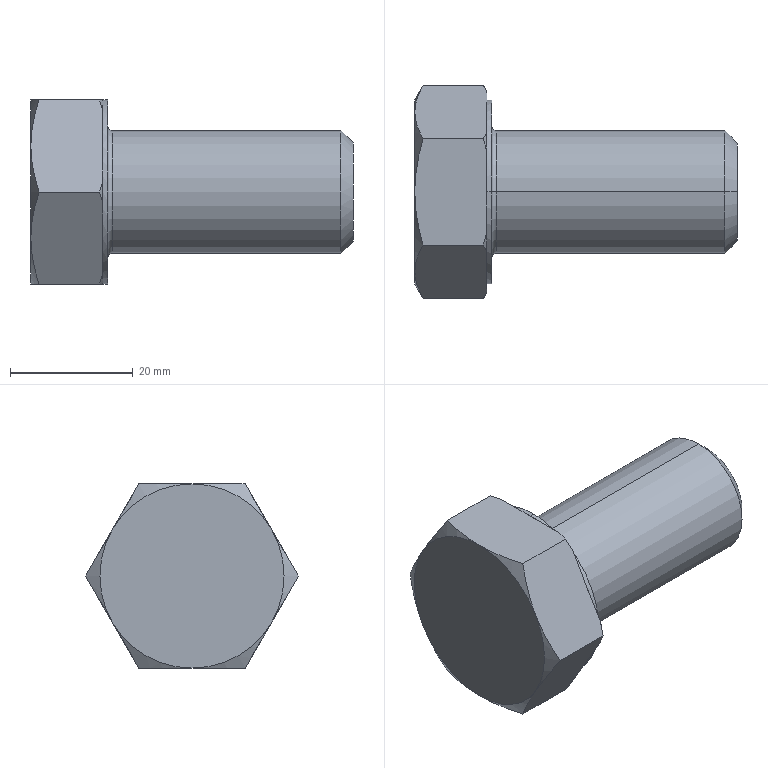Part | SolidWorks | 1 solid | 35 faces | box 52.5 x 34.641 x 30 mm | volume 22112 mm3 | plane 15 | cone 14 | cylinder 4 | torus 2 | commonest cylinder face diameters 20 x2 30 x2
STEP:
#1=CARTESIAN_POINT('',(13.3,0.,10.));
#2=VERTEX_POINT('',#1);
#3=CARTESIAN_POINT('',(13.3,0.,-10.));
#4=VERTEX_POINT('',#3);
#5=CARTESIAN_POINT('',(13.3,0.,0.));
#6=DIRECTION('',(1.,0.,0.));
#7=DIRECTION('',(0.,0.,-1.));
#8=AXIS2_PLACEMENT_3D('',#5,#6,#7);
#9=CIRCLE('',#8,10.);
#10=EDGE_CURVE('',#2,#4,#9,.T.);
#11=ORIENTED_EDGE('',*,*,#10,.F.);
#12=CARTESIAN_POINT('',(12.5,0.,10.8));
#13=VERTEX_POINT('',#12);
#14=CARTESIAN_POINT('',(13.3,0.,10.8));
#15=DIRECTION('',(0.,1.,0.));
#16=DIRECTION('',(0.,0.,1.));
#17=AXIS2_PLACEMENT_3D('',#14,#15,#16);
#18=CIRCLE('',#17,0.8);
#19=EDGE_CURVE('',#2,#13,#18,.T.);
#20=ORIENTED_EDGE('',*,*,#19,.T.);
#21=CARTESIAN_POINT('',(12.5,0.,-10.8));
#22=VERTEX_POINT('',#21);
#23=CARTESIAN_POINT('',(12.5,0.,0.));
#24=DIRECTION('',(-1.,0.,0.));
#25=DIRECTION('',(0.,0.,-1.));
#26=AXIS2_PLACEMENT_3D('',#23,#24,#25);
#27=CIRCLE('',#26,10.8);
#28=EDGE_CURVE('',#22,#13,#27,.T.);
#29=ORIENTED_EDGE('',*,*,#28,.F.);
#30=CARTESIAN_POINT('',(13.3,0.,-10.8));
#31=DIRECTION('',(0.,-1.,0.));
#32=DIRECTION('',(0.,0.,-1.));
#33=AXIS2_PLACEMENT_3D('',#30,#31,#32);
#34=CIRCLE('',#33,0.8);
#35=EDGE_CURVE('',#4,#22,#34,.T.);
#36=ORIENTED_EDGE('',*,*,#35,.F.);
#37=EDGE_LOOP('',(#11,#20,#29,#36));
#38=FACE_OUTER_BOUND('',#37,.T.);
#39=CARTESIAN_POINT('',(13.3,0.,0.));
#40=DIRECTION('',(1.,0.,0.));
#41=DIRECTION('',(0.,0.,-1.));
#42=AXIS2_PLACEMENT_3D('',#39,#40,#41);
#43=TOROIDAL_SURFACE('',#42,10.8,0.8);
#44=ADVANCED_FACE('',(#38),#43,.F.);
#45=CARTESIAN_POINT('',(52.5,0.,-8.));
#46=VERTEX_POINT('',#45);
#47=CARTESIAN_POINT('',(52.5,0.,8.));
#48=VERTEX_POINT('',#47);
#49=CARTESIAN_POINT('',(52.5,0.,0.));
#50=DIRECTION('',(1.,0.,0.));
#51=DIRECTION('',(0.,0.,1.));
#52=AXIS2_PLACEMENT_3D('',#49,#50,#51);
#53=CIRCLE('',#52,8.);
#54=EDGE_CURVE('',#46,#48,#53,.T.);
#55=ORIENTED_EDGE('',*,*,#54,.F.);
#56=CARTESIAN_POINT('',(50.5,0.,-10.));
#57=VERTEX_POINT('',#56);
#58=CARTESIAN_POINT('',(50.5,0.,-10.));
#59=DIRECTION('',(-0.7071,0.,-0.7071));
#60=VECTOR('',#59,1000.);
#61=LINE('',#58,#60);
#62=EDGE_CURVE('',#46,#57,#61,.T.);
#63=ORIENTED_EDGE('',*,*,#62,.T.);
#64=CARTESIAN_POINT('',(50.5,0.,10.));
#65=VERTEX_POINT('',#64);
#66=CARTESIAN_POINT('',(50.5,0.,0.));
#67=DIRECTION('',(-1.,0.,0.));
#68=DIRECTION('',(0.,0.,1.));
#69=AXIS2_PLACEMENT_3D('',#66,#67,#68);
#70=CIRCLE('',#69,10.);
#71=EDGE_CURVE('',#65,#57,#70,.T.);
#72=ORIENTED_EDGE('',*,*,#71,.F.);
#73=CARTESIAN_POINT('',(50.5,0.,10.));
#74=DIRECTION('',(-0.7071,0.,0.7071));
#75=VECTOR('',#74,1000.);
#76=LINE('',#73,#75);
#77=EDGE_CURVE('',#48,#65,#76,.T.);
#78=ORIENTED_EDGE('',*,*,#77,.F.);
#79=EDGE_LOOP('',(#55,#63,#72,#78));
#80=FACE_OUTER_BOUND('',#79,.T.);
#81=CARTESIAN_POINT('',(50.5,0.,0.));
#82=DIRECTION('',(-1.,0.,0.));
#83=DIRECTION('',(0.,0.,1.));
#84=AXIS2_PLACEMENT_3D('',#81,#82,#83);
#85=CONICAL_SURFACE('',#84,10.,0.7854);
#86=ADVANCED_FACE('',(#80),#85,.T.);
#87=ORIENTED_EDGE('',*,*,#71,.T.);
#88=CARTESIAN_POINT('',(0.,0.,-10.));
#89=DIRECTION('',(-1.,0.,0.));
#90=VECTOR('',#89,1000.);
#91=LINE('',#88,#90);
#92=EDGE_CURVE('',#57,#4,#91,.T.);
#93=ORIENTED_EDGE('',*,*,#92,.T.);
#94=CARTESIAN_POINT('',(13.3,0.,0.));
#95=DIRECTION('',(1.,0.,0.));
#96=DIRECTION('',(0.,0.,-1.));
#97=AXIS2_PLACEMENT_3D('',#94,#95,#96);
#98=CIRCLE('',#97,10.);
#99=EDGE_CURVE('',#4,#2,#98,.T.);
#100=ORIENTED_EDGE('',*,*,#99,.T.);
#101=CARTESIAN_POINT('',(0.,0.,10.));
#102=DIRECTION('',(-1.,0.,0.));
#103=VECTOR('',#102,1000.);
#104=LINE('',#101,#103);
#105=EDGE_CURVE('',#65,#2,#104,.T.);
#106=ORIENTED_EDGE('',*,*,#105,.F.);
#107=EDGE_LOOP('',(#87,#93,#100,#106));
#108=FACE_OUTER_BOUND('',#107,.T.);
#109=CARTESIAN_POINT('',(0.,0.,0.));
#110=DIRECTION('',(-1.,0.,0.));
#111=DIRECTION('',(0.,0.,1.));
#112=AXIS2_PLACEMENT_3D('',#109,#110,#111);
#113=CYLINDRICAL_SURFACE('',#112,10.);
#114=ADVANCED_FACE('',(#108),#113,.T.);
#115=CARTESIAN_POINT('',(12.5,0.,-15.));
#116=VERTEX_POINT('',#115);
#117=CARTESIAN_POINT('',(12.5,0.,15.));
#118=VERTEX_POINT('',#117);
#119=CARTESIAN_POINT('',(12.5,0.,0.));
#120=DIRECTION('',(1.,0.,0.));
#121=DIRECTION('',(0.,0.,-1.));
#122=AXIS2_PLACEMENT_3D('',#119,#120,#121);
#123=CIRCLE('',#122,15.);
#124=EDGE_CURVE('',#116,#118,#123,.T.);
#125=ORIENTED_EDGE('',*,*,#124,.F.);
#126=CARTESIAN_POINT('',(11.7,0.,-15.));
#127=VERTEX_POINT('',#126);
#128=CARTESIAN_POINT('',(0.,0.,-15.));
#129=DIRECTION('',(-1.,0.,0.));
#130=VECTOR('',#129,1000.);
#131=LINE('',#128,#130);
#132=EDGE_CURVE('',#116,#127,#131,.T.);
#133=ORIENTED_EDGE('',*,*,#132,.T.);
#134=CARTESIAN_POINT('',(11.7,12.99,-7.5));
#135=VERTEX_POINT('',#134);
#136=CARTESIAN_POINT('',(11.7,0.,0.));
#137=DIRECTION('',(-1.,0.,0.));
#138=DIRECTION('',(0.,0.,1.));
#139=AXIS2_PLACEMENT_3D('',#136,#137,#138);
#140=CIRCLE('',#139,15.);
#141=EDGE_CURVE('',#135,#127,#140,.T.);
#142=ORIENTED_EDGE('',*,*,#141,.F.);
#143=CARTESIAN_POINT('',(11.7,12.99,7.5));
#144=VERTEX_POINT('',#143);
#145=CARTESIAN_POINT('',(11.7,0.,0.));
#146=DIRECTION('',(-1.,0.,0.));
#147=DIRECTION('',(0.,0.,1.));
#148=AXIS2_PLACEMENT_3D('',#145,#146,#147);
#149=CIRCLE('',#148,15.);
#150=EDGE_CURVE('',#144,#135,#149,.T.);
#151=ORIENTED_EDGE('',*,*,#150,.F.);
#152=CARTESIAN_POINT('',(11.7,0.,15.));
#153=VERTEX_POINT('',#152);
#154=CARTESIAN_POINT('',(11.7,0.,0.));
#155=DIRECTION('',(-1.,0.,0.));
#156=DIRECTION('',(0.,0.,1.));
#157=AXIS2_PLACEMENT_3D('',#154,#155,#156);
#158=CIRCLE('',#157,15.);
#159=EDGE_CURVE('',#153,#144,#158,.T.);
#160=ORIENTED_EDGE('',*,*,#159,.F.);
#161=CARTESIAN_POINT('',(0.,0.,15.));
#162=DIRECTION('',(-1.,0.,0.));
#163=VECTOR('',#162,1000.);
#164=LINE('',#161,#163);
#165=EDGE_CURVE('',#118,#153,#164,.T.);
#166=ORIENTED_EDGE('',*,*,#165,.F.);
#167=EDGE_LOOP('',(#125,#133,#142,#151,#160,#166));
#168=FACE_OUTER_BOUND('',#167,.T.);
#169=CARTESIAN_POINT('',(0.,0.,0.));
#170=DIRECTION('',(-1.,0.,0.));
#171=DIRECTION('',(0.,0.,1.));
#172=AXIS2_PLACEMENT_3D('',#169,#170,#171);
#173=CYLINDRICAL_SURFACE('',#172,15.);
#174=ADVANCED_FACE('',(#168),#173,.T.);
#175=CARTESIAN_POINT('',(11.7,9.693,-13.211));
#176=VERTEX_POINT('',#175);
#177=CARTESIAN_POINT('',(11.7,8.66,-15.));
#178=DIRECTION('',(0.,0.5,0.866));
#179=VECTOR('',#178,1000.);
#180=LINE('',#177,#179);
#181=EDGE_CURVE('',#176,#135,#180,.T.);
#182=ORIENTED_EDGE('',*,*,#181,.F.);
#183=CARTESIAN_POINT('',(11.16,8.66,-15.));
#184=VERTEX_POINT('',#183);
#185=CARTESIAN_POINT('',(11.16,8.66,-15.));
#186=CARTESIAN_POINT('',(11.358,9.003,-14.406));
#187=CARTESIAN_POINT('',(11.539,9.347,-13.81));
#188=CARTESIAN_POINT('',(11.7,9.693,-13.211));
#189=B_SPLINE_CURVE_WITH_KNOTS('',3,(#185,#186,#187,#188),.UNSPECIFIED.,.F.,.F.,(4,4),(0.000000238,0.002122),.UNSPECIFIED.);
#190=EDGE_CURVE('',#184,#176,#189,.T.);
#191=ORIENTED_EDGE('',*,*,#190,.F.);
#192=CARTESIAN_POINT('',(1.34,8.66,-15.));
#193=VERTEX_POINT('',#192);
#194=CARTESIAN_POINT('',(12.5,8.66,-15.));
#195=DIRECTION('',(-1.,0.,0.));
#196=VECTOR('',#195,1000.);
#197=LINE('',#194,#196);
#198=EDGE_CURVE('',#184,#193,#197,.T.);
#199=ORIENTED_EDGE('',*,*,#198,.T.);
#200=CARTESIAN_POINT('',(0.,12.99,-7.5));
#201=VERTEX_POINT('',#200);
#202=CARTESIAN_POINT('',(0.,12.99,-7.5));
#203=CARTESIAN_POINT('',(0.,12.623,-8.136));
#204=CARTESIAN_POINT('',(0.03167,12.254,-8.776));
#205=CARTESIAN_POINT('',(0.1542,11.524,-10.041));
#206=CARTESIAN_POINT('',(0.245,11.161,-10.669));
#207=CARTESIAN_POINT('',(0.595,10.079,-12.542));
#208=CARTESIAN_POINT('',(0.9318,9.367,-13.776));
#209=CARTESIAN_POINT('',(1.34,8.66,-15.));
#210=B_SPLINE_CURVE_WITH_KNOTS('',3,(#202,#203,#204,#205,#206,#207,#208,#209),.UNSPECIFIED.,.F.,.F.,(4,2,2,4),(0.008763,0.01095,0.01313,0.01749),.UNSPECIFIED.);
#211=EDGE_CURVE('',#201,#193,#210,.T.);
#212=ORIENTED_EDGE('',*,*,#211,.F.);
#213=CARTESIAN_POINT('',(1.34,17.321,0.));
#214=VERTEX_POINT('',#213);
#215=CARTESIAN_POINT('',(1.34,17.321,0.));
#216=CARTESIAN_POINT('',(0.9308,16.612,-1.227));
#217=CARTESIAN_POINT('',(0.5939,15.899,-2.463));
#218=CARTESIAN_POINT('',(0.1277,14.457,-4.96));
#219=CARTESIAN_POINT('',(0.,13.728,-6.222));
#220=CARTESIAN_POINT('',(0.,12.99,-7.5));
#221=B_SPLINE_CURVE_WITH_KNOTS('',3,(#215,#216,#217,#218,#219,#220),.UNSPECIFIED.,.F.,.F.,(4,2,4),(0.000000238,0.004382,0.008763),.UNSPECIFIED.);
#222=EDGE_CURVE('',#214,#201,#221,.T.);
#223=ORIENTED_EDGE('',*,*,#222,.F.);
#224=CARTESIAN_POINT('',(11.16,17.321,0.));
#225=VERTEX_POINT('',#224);
#226=CARTESIAN_POINT('',(12.5,17.321,0.));
#227=DIRECTION('',(-1.,0.,0.));
#228=VECTOR('',#227,1000.);
#229=LINE('',#226,#228);
#230=EDGE_CURVE('',#225,#214,#229,.T.);
#231=ORIENTED_EDGE('',*,*,#230,.F.);
#232=CARTESIAN_POINT('',(11.7,16.288,-1.789));
#233=VERTEX_POINT('',#232);
#234=CARTESIAN_POINT('',(11.7,16.288,-1.789));
#235=CARTESIAN_POINT('',(11.539,16.634,-1.19));
#236=CARTESIAN_POINT('',(11.358,16.978,-0.5937));
#237=CARTESIAN_POINT('',(11.16,17.321,0.));
#238=B_SPLINE_CURVE_WITH_KNOTS('',3,(#234,#235,#236,#237),.UNSPECIFIED.,.F.,.F.,(4,4),(0.01538,0.01749),.UNSPECIFIED.);
#239=EDGE_CURVE('',#233,#225,#238,.T.);
#240=ORIENTED_EDGE('',*,*,#239,.F.);
#241=CARTESIAN_POINT('',(11.7,8.66,-15.));
#242=DIRECTION('',(0.,0.5,0.866));
#243=VECTOR('',#242,1000.);
#244=LINE('',#241,#243);
#245=EDGE_CURVE('',#135,#233,#244,.T.);
#246=ORIENTED_EDGE('',*,*,#245,.F.);
#247=EDGE_LOOP('',(#182,#191,#199,#212,#223,#231,#240,#246));
#248=FACE_OUTER_BOUND('',#247,.T.);
#249=CARTESIAN_POINT('',(12.5,8.66,-15.));
#250=DIRECTION('',(0.,-0.866,0.5));
#251=DIRECTION('',(0.,-0.5,-0.866));
#252=AXIS2_PLACEMENT_3D('',#249,#250,#251);
#253=PLANE('',#252);
#254=ADVANCED_FACE('',(#248),#253,.F.);
#255=CARTESIAN_POINT('',(11.7,16.288,1.789));
#256=VERTEX_POINT('',#255);
#257=CARTESIAN_POINT('',(11.7,17.321,0.));
#258=DIRECTION('',(0.,-0.5,0.866));
#259=VECTOR('',#258,1000.);
#260=LINE('',#257,#259);
#261=EDGE_CURVE('',#256,#144,#260,.T.);
#262=ORIENTED_EDGE('',*,*,#261,.F.);
#263=CARTESIAN_POINT('',(11.16,17.321,0.));
#264=CARTESIAN_POINT('',(11.358,16.978,0.594));
#265=CARTESIAN_POINT('',(11.539,16.633,1.19));
#266=CARTESIAN_POINT('',(11.7,16.288,1.789));
#267=B_SPLINE_CURVE_WITH_KNOTS('',3,(#263,#264,#265,#266),.UNSPECIFIED.,.F.,.F.,(4,4),(0.000000238,0.002122),.UNSPECIFIED.);
#268=EDGE_CURVE('',#225,#256,#267,.T.);
#269=ORIENTED_EDGE('',*,*,#268,.F.);
#270=ORIENTED_EDGE('',*,*,#230,.T.);
#271=CARTESIAN_POINT('',(0.,12.99,7.5));
#272=VERTEX_POINT('',#271);
#273=CARTESIAN_POINT('',(0.,12.99,7.5));
#274=CARTESIAN_POINT('',(0.,13.358,6.864));
#275=CARTESIAN_POINT('',(0.03167,13.727,6.224));
#276=CARTESIAN_POINT('',(0.1542,14.457,4.959));
#277=CARTESIAN_POINT('',(0.245,14.82,4.331));
#278=CARTESIAN_POINT('',(0.595,15.901,2.458));
#279=CARTESIAN_POINT('',(0.9318,16.614,1.224));
#280=CARTESIAN_POINT('',(1.34,17.321,0.));
#281=B_SPLINE_CURVE_WITH_KNOTS('',3,(#273,#274,#275,#276,#277,#278,#279,#280),.UNSPECIFIED.,.F.,.F.,(4,2,2,4),(0.008763,0.01095,0.01313,0.01749),.UNSPECIFIED.);
#282=EDGE_CURVE('',#272,#214,#281,.T.);
#283=ORIENTED_EDGE('',*,*,#282,.F.);
#284=CARTESIAN_POINT('',(1.34,8.66,15.));
#285=VERTEX_POINT('',#284);
#286=CARTESIAN_POINT('',(1.34,8.66,15.));
#287=CARTESIAN_POINT('',(0.9308,9.369,13.773));
#288=CARTESIAN_POINT('',(0.5939,10.082,12.537));
#289=CARTESIAN_POINT('',(0.1277,11.524,10.04));
#290=CARTESIAN_POINT('',(0.,12.253,8.778));
#291=CARTESIAN_POINT('',(0.,12.99,7.5));
#292=B_SPLINE_CURVE_WITH_KNOTS('',3,(#286,#287,#288,#289,#290,#291),.UNSPECIFIED.,.F.,.F.,(4,2,4),(0.000000238,0.004382,0.008763),.UNSPECIFIED.);
#293=EDGE_CURVE('',#285,#272,#292,.T.);
#294=ORIENTED_EDGE('',*,*,#293,.F.);
#295=CARTESIAN_POINT('',(11.16,8.66,15.));
#296=VERTEX_POINT('',#295);
#297=CARTESIAN_POINT('',(12.5,8.66,15.));
#298=DIRECTION('',(-1.,0.,0.));
#299=VECTOR('',#298,1000.);
#300=LINE('',#297,#299);
#301=EDGE_CURVE('',#296,#285,#300,.T.);
#302=ORIENTED_EDGE('',*,*,#301,.F.);
#303=CARTESIAN_POINT('',(11.7,9.693,13.211));
#304=VERTEX_POINT('',#303);
#305=CARTESIAN_POINT('',(11.7,9.693,13.211));
#306=CARTESIAN_POINT('',(11.539,9.347,13.81));
#307=CARTESIAN_POINT('',(11.358,9.003,14.406));
#308=CARTESIAN_POINT('',(11.16,8.66,15.));
#309=B_SPLINE_CURVE_WITH_KNOTS('',3,(#305,#306,#307,#308),.UNSPECIFIED.,.F.,.F.,(4,4),(0.01538,0.01749),.UNSPECIFIED.);
#310=EDGE_CURVE('',#304,#296,#309,.T.);
#311=ORIENTED_EDGE('',*,*,#310,.F.);
#312=CARTESIAN_POINT('',(11.7,17.321,0.));
#313=DIRECTION('',(0.,-0.5,0.866));
#314=VECTOR('',#313,1000.);
#315=LINE('',#312,#314);
#316=EDGE_CURVE('',#144,#304,#315,.T.);
#317=ORIENTED_EDGE('',*,*,#316,.F.);
#318=EDGE_LOOP('',(#262,#269,#270,#283,#294,#302,#311,#317));
#319=FACE_OUTER_BOUND('',#318,.T.);
#320=CARTESIAN_POINT('',(12.5,17.321,0.));
#321=DIRECTION('',(0.,-0.866,-0.5));
#322=DIRECTION('',(0.,0.5,-0.866));
#323=AXIS2_PLACEMENT_3D('',#320,#321,#322);
#324=PLANE('',#323);
#325=ADVANCED_FACE('',(#319),#324,.F.);
#326=CARTESIAN_POINT('',(11.7,6.595,15.));
#327=VERTEX_POINT('',#326);
#328=CARTESIAN_POINT('',(11.7,8.66,15.));
#329=DIRECTION('',(0.,-1.,0.));
#330=VECTOR('',#329,1000.);
#331=LINE('',#328,#330);
#332=EDGE_CURVE('',#327,#153,#331,.T.);
#333=ORIENTED_EDGE('',*,*,#332,.F.);
#334=CARTESIAN_POINT('',(11.16,8.66,15.));
#335=CARTESIAN_POINT('',(11.358,7.976,15.));
#336=CARTESIAN_POINT('',(11.539,7.288,15.));
#337=CARTESIAN_POINT('',(11.7,6.595,15.));
#338=B_SPLINE_CURVE_WITH_KNOTS('',3,(#334,#335,#336,#337),.UNSPECIFIED.,.F.,.F.,(4,4),(0.03969,0.04183),.UNSPECIFIED.);
#339=EDGE_CURVE('',#296,#327,#338,.T.);
#340=ORIENTED_EDGE('',*,*,#339,.F.);
#341=ORIENTED_EDGE('',*,*,#301,.T.);
#342=CARTESIAN_POINT('',(0.,0.,15.));
#343=VERTEX_POINT('',#342);
#344=CARTESIAN_POINT('',(0.,0.,15.));
#345=CARTESIAN_POINT('',(0.,0.7329,15.));
#346=CARTESIAN_POINT('',(0.03126,1.469,15.));
#347=CARTESIAN_POINT('',(0.1552,2.944,15.));
#348=CARTESIAN_POINT('',(0.2469,3.673,15.));
#349=CARTESIAN_POINT('',(0.5989,5.841,15.));
#350=CARTESIAN_POINT('',(0.9354,7.26,15.));
#351=CARTESIAN_POINT('',(1.34,8.66,15.));
#352=B_SPLINE_CURVE_WITH_KNOTS('',3,(#344,#345,#346,#347,#348,#349,#350,#351),.UNSPECIFIED.,.F.,.F.,(4,2,2,4),(0.02466,0.02686,0.02905,0.03344),.UNSPECIFIED.);
#353=EDGE_CURVE('',#343,#285,#352,.T.);
#354=ORIENTED_EDGE('',*,*,#353,.F.);
#355=CARTESIAN_POINT('',(1.34,-8.66,15.));
#356=VERTEX_POINT('',#355);
#357=CARTESIAN_POINT('',(1.34,-8.66,15.));
#358=CARTESIAN_POINT('',(0.9328,-7.25,15.));
#359=CARTESIAN_POINT('',(0.592,-5.808,15.));
#360=CARTESIAN_POINT('',(0.126,-2.919,15.));
#361=CARTESIAN_POINT('',(0.,-1.465,15.));
#362=CARTESIAN_POINT('',(0.,0.,15.));
#363=B_SPLINE_CURVE_WITH_KNOTS('',3,(#357,#358,#359,#360,#361,#362),.UNSPECIFIED.,.F.,.F.,(4,2,4),(0.0159,0.02028,0.02466),.UNSPECIFIED.);
#364=EDGE_CURVE('',#356,#343,#363,.T.);
#365=ORIENTED_EDGE('',*,*,#364,.F.);
#366=CARTESIAN_POINT('',(11.16,-8.66,15.));
#367=VERTEX_POINT('',#366);
#368=CARTESIAN_POINT('',(12.5,-8.66,15.));
#369=DIRECTION('',(-1.,0.,0.));
#370=VECTOR('',#369,1000.);
#371=LINE('',#368,#370);
#372=EDGE_CURVE('',#367,#356,#371,.T.);
#373=ORIENTED_EDGE('',*,*,#372,.F.);
#374=CARTESIAN_POINT('',(11.7,-6.595,15.));
#375=VERTEX_POINT('',#374);
#376=CARTESIAN_POINT('',(11.7,-6.595,15.));
#377=CARTESIAN_POINT('',(11.539,-7.289,15.));
#378=CARTESIAN_POINT('',(11.357,-7.978,15.));
#379=CARTESIAN_POINT('',(11.16,-8.66,15.));
#380=B_SPLINE_CURVE_WITH_KNOTS('',3,(#376,#377,#378,#379),.UNSPECIFIED.,.F.,.F.,(4,4),(0.05511,0.05723),.UNSPECIFIED.);
#381=EDGE_CURVE('',#375,#367,#380,.T.);
#382=ORIENTED_EDGE('',*,*,#381,.F.);
#383=CARTESIAN_POINT('',(11.7,8.66,15.));
#384=DIRECTION('',(0.,-1.,0.));
#385=VECTOR('',#384,1000.);
#386=LINE('',#383,#385);
#387=EDGE_CURVE('',#153,#375,#386,.T.);
#388=ORIENTED_EDGE('',*,*,#387,.F.);
#389=EDGE_LOOP('',(#333,#340,#341,#354,#365,#373,#382,#388));
#390=FACE_OUTER_BOUND('',#389,.T.);
#391=CARTESIAN_POINT('',(12.5,8.66,15.));
#392=DIRECTION('',(0.,0.,-1.));
#393=DIRECTION('',(0.,1.,0.));
#394=AXIS2_PLACEMENT_3D('',#391,#392,#393);
#395=PLANE('',#394);
#396=ADVANCED_FACE('',(#390),#395,.F.);
#397=CARTESIAN_POINT('',(11.7,-9.693,13.211));
#398=VERTEX_POINT('',#397);
#399=CARTESIAN_POINT('',(11.7,-12.99,7.5));
#400=VERTEX_POINT('',#399);
#401=CARTESIAN_POINT('',(11.7,-17.321,0.));
#402=DIRECTION('',(0.,-0.5,-0.866));
#403=VECTOR('',#402,1000.);
#404=LINE('',#401,#403);
#405=EDGE_CURVE('',#398,#400,#404,.T.);
#406=ORIENTED_EDGE('',*,*,#405,.F.);
#407=CARTESIAN_POINT('',(11.16,-8.66,15.));
#408=CARTESIAN_POINT('',(11.358,-9.003,14.406));
#409=CARTESIAN_POINT('',(11.539,-9.347,13.81));
#410=CARTESIAN_POINT('',(11.7,-9.693,13.211));
#411=B_SPLINE_CURVE_WITH_KNOTS('',3,(#407,#408,#409,#410),.UNSPECIFIED.,.F.,.F.,(4,4),(0.000000238,0.002122),.UNSPECIFIED.);
#412=EDGE_CURVE('',#367,#398,#411,.T.);
#413=ORIENTED_EDGE('',*,*,#412,.F.);
#414=ORIENTED_EDGE('',*,*,#372,.T.);
#415=CARTESIAN_POINT('',(0.,-12.99,7.5));
#416=VERTEX_POINT('',#415);
#417=CARTESIAN_POINT('',(0.,-12.99,7.5));
#418=CARTESIAN_POINT('',(0.,-12.623,8.136));
#419=CARTESIAN_POINT('',(0.03167,-12.254,8.776));
#420=CARTESIAN_POINT('',(0.1542,-11.524,10.041));
#421=CARTESIAN_POINT('',(0.245,-11.161,10.669));
#422=CARTESIAN_POINT('',(0.595,-10.079,12.542));
#423=CARTESIAN_POINT('',(0.9318,-9.367,13.776));
#424=CARTESIAN_POINT('',(1.34,-8.66,15.));
#425=B_SPLINE_CURVE_WITH_KNOTS('',3,(#417,#418,#419,#420,#421,#422,#423,#424),.UNSPECIFIED.,.F.,.F.,(4,2,2,4),(0.008763,0.01095,0.01313,0.01749),.UNSPECIFIED.);
#426=EDGE_CURVE('',#416,#356,#425,.T.);
#427=ORIENTED_EDGE('',*,*,#426,.F.);
#428=CARTESIAN_POINT('',(1.34,-17.321,0.));
#429=VERTEX_POINT('',#428);
#430=CARTESIAN_POINT('',(1.34,-17.321,0.));
#431=CARTESIAN_POINT('',(0.9308,-16.612,1.227));
#432=CARTESIAN_POINT('',(0.5939,-15.899,2.463));
#433=CARTESIAN_POINT('',(0.1277,-14.457,4.96));
#434=CARTESIAN_POINT('',(0.,-13.728,6.222));
#435=CARTESIAN_POINT('',(0.,-12.99,7.5));
#436=B_SPLINE_CURVE_WITH_KNOTS('',3,(#430,#431,#432,#433,#434,#435),.UNSPECIFIED.,.F.,.F.,(4,2,4),(0.000000238,0.004382,0.008763),.UNSPECIFIED.);
#437=EDGE_CURVE('',#429,#416,#436,.T.);
#438=ORIENTED_EDGE('',*,*,#437,.F.);
#439=CARTESIAN_POINT('',(11.16,-17.321,0.));
#440=VERTEX_POINT('',#439);
#441=CARTESIAN_POINT('',(12.5,-17.321,0.));
#442=DIRECTION('',(-1.,0.,0.));
#443=VECTOR('',#442,1000.);
#444=LINE('',#441,#443);
#445=EDGE_CURVE('',#440,#429,#444,.T.);
#446=ORIENTED_EDGE('',*,*,#445,.F.);
#447=CARTESIAN_POINT('',(11.7,-16.288,1.789));
#448=VERTEX_POINT('',#447);
#449=CARTESIAN_POINT('',(11.7,-16.288,1.789));
#450=CARTESIAN_POINT('',(11.539,-16.634,1.19));
#451=CARTESIAN_POINT('',(11.358,-16.978,0.5937));
#452=CARTESIAN_POINT('',(11.16,-17.321,0.));
#453=B_SPLINE_CURVE_WITH_KNOTS('',3,(#449,#450,#451,#452),.UNSPECIFIED.,.F.,.F.,(4,4),(0.01538,0.01749),.UNSPECIFIED.);
#454=EDGE_CURVE('',#448,#440,#453,.T.);
#455=ORIENTED_EDGE('',*,*,#454,.F.);
#456=CARTESIAN_POINT('',(11.7,-17.321,0.));
#457=DIRECTION('',(0.,-0.5,-0.866));
#458=VECTOR('',#457,1000.);
#459=LINE('',#456,#458);
#460=EDGE_CURVE('',#400,#448,#459,.T.);
#461=ORIENTED_EDGE('',*,*,#460,.F.);
#462=EDGE_LOOP('',(#406,#413,#414,#427,#438,#446,#455,#461));
#463=FACE_OUTER_BOUND('',#462,.T.);
#464=CARTESIAN_POINT('',(12.5,-17.321,0.));
#465=DIRECTION('',(0.,0.866,-0.5));
#466=DIRECTION('',(0.,0.5,0.866));
#467=AXIS2_PLACEMENT_3D('',#464,#465,#466);
#468=PLANE('',#467);
#469=ADVANCED_FACE('',(#463),#468,.F.);
#470=CARTESIAN_POINT('',(11.7,-16.288,-1.789));
#471=VERTEX_POINT('',#470);
#472=CARTESIAN_POINT('',(11.7,-12.99,-7.5));
#473=VERTEX_POINT('',#472);
#474=CARTESIAN_POINT('',(11.7,-8.66,-15.));
#475=DIRECTION('',(0.,0.5,-0.866));
#476=VECTOR('',#475,1000.);
#477=LINE('',#474,#476);
#478=EDGE_CURVE('',#471,#473,#477,.T.);
#479=ORIENTED_EDGE('',*,*,#478,.F.);
#480=CARTESIAN_POINT('',(11.16,-17.321,0.));
#481=CARTESIAN_POINT('',(11.358,-16.978,-0.594));
#482=CARTESIAN_POINT('',(11.539,-16.633,-1.19));
#483=CARTESIAN_POINT('',(11.7,-16.288,-1.789));
#484=B_SPLINE_CURVE_WITH_KNOTS('',3,(#480,#481,#482,#483),.UNSPECIFIED.,.F.,.F.,(4,4),(0.000000238,0.002122),.UNSPECIFIED.);
#485=EDGE_CURVE('',#440,#471,#484,.T.);
#486=ORIENTED_EDGE('',*,*,#485,.F.);
#487=ORIENTED_EDGE('',*,*,#445,.T.);
#488=CARTESIAN_POINT('',(0.,-12.99,-7.5));
#489=VERTEX_POINT('',#488);
#490=CARTESIAN_POINT('',(0.,-12.99,-7.5));
#491=CARTESIAN_POINT('',(0.,-13.358,-6.864));
#492=CARTESIAN_POINT('',(0.03167,-13.727,-6.224));
#493=CARTESIAN_POINT('',(0.1542,-14.457,-4.959));
#494=CARTESIAN_POINT('',(0.245,-14.82,-4.331));
#495=CARTESIAN_POINT('',(0.595,-15.901,-2.458));
#496=CARTESIAN_POINT('',(0.9318,-16.614,-1.224));
#497=CARTESIAN_POINT('',(1.34,-17.321,0.));
#498=B_SPLINE_CURVE_WITH_KNOTS('',3,(#490,#491,#492,#493,#494,#495,#496,#497),.UNSPECIFIED.,.F.,.F.,(4,2,2,4),(0.008763,0.01095,0.01313,0.01749),.UNSPECIFIED.);
#499=EDGE_CURVE('',#489,#429,#498,.T.);
#500=ORIENTED_EDGE('',*,*,#499,.F.);
#501=CARTESIAN_POINT('',(1.34,-8.66,-15.));
#502=VERTEX_POINT('',#501);
#503=CARTESIAN_POINT('',(1.34,-8.66,-15.));
#504=CARTESIAN_POINT('',(0.9308,-9.369,-13.773));
#505=CARTESIAN_POINT('',(0.5939,-10.082,-12.537));
#506=CARTESIAN_POINT('',(0.1277,-11.524,-10.04));
#507=CARTESIAN_POINT('',(0.,-12.253,-8.778));
#508=CARTESIAN_POINT('',(0.,-12.99,-7.5));
#509=B_SPLINE_CURVE_WITH_KNOTS('',3,(#503,#504,#505,#506,#507,#508),.UNSPECIFIED.,.F.,.F.,(4,2,4),(0.000000238,0.004382,0.008763),.UNSPECIFIED.);
#510=EDGE_CURVE('',#502,#489,#509,.T.);
#511=ORIENTED_EDGE('',*,*,#510,.F.);
#512=CARTESIAN_POINT('',(11.16,-8.66,-15.));
#513=VERTEX_POINT('',#512);
#514=CARTESIAN_POINT('',(12.5,-8.66,-15.));
#515=DIRECTION('',(-1.,0.,0.));
#516=VECTOR('',#515,1000.);
#517=LINE('',#514,#516);
#518=EDGE_CURVE('',#513,#502,#517,.T.);
#519=ORIENTED_EDGE('',*,*,#518,.F.);
#520=CARTESIAN_POINT('',(11.7,-9.693,-13.211));
#521=VERTEX_POINT('',#520);
#522=CARTESIAN_POINT('',(11.7,-9.693,-13.211));
#523=CARTESIAN_POINT('',(11.539,-9.347,-13.81));
#524=CARTESIAN_POINT('',(11.358,-9.003,-14.406));
#525=CARTESIAN_POINT('',(11.16,-8.66,-15.));
#526=B_SPLINE_CURVE_WITH_KNOTS('',3,(#522,#523,#524,#525),.UNSPECIFIED.,.F.,.F.,(4,4),(0.01538,0.01749),.UNSPECIFIED.);
#527=EDGE_CURVE('',#521,#513,#526,.T.);
#528=ORIENTED_EDGE('',*,*,#527,.F.);
#529=CARTESIAN_POINT('',(11.7,-8.66,-15.));
#530=DIRECTION('',(0.,0.5,-0.866));
#531=VECTOR('',#530,1000.);
#532=LINE('',#529,#531);
#533=EDGE_CURVE('',#473,#521,#532,.T.);
#534=ORIENTED_EDGE('',*,*,#533,.F.);
#535=EDGE_LOOP('',(#479,#486,#487,#500,#511,#519,#528,#534));
#536=FACE_OUTER_BOUND('',#535,.T.);
#537=CARTESIAN_POINT('',(12.5,-8.66,-15.));
#538=DIRECTION('',(0.,0.866,0.5));
#539=DIRECTION('',(0.,-0.5,0.866));
#540=AXIS2_PLACEMENT_3D('',#537,#538,#539);
#541=PLANE('',#540);
#542=ADVANCED_FACE('',(#536),#541,.F.);
#543=CARTESIAN_POINT('',(11.7,-6.595,-15.));
#544=VERTEX_POINT('',#543);
#545=CARTESIAN_POINT('',(11.7,8.66,-15.));
#546=DIRECTION('',(0.,1.,0.));
#547=VECTOR('',#546,1000.);
#548=LINE('',#545,#547);
#549=EDGE_CURVE('',#544,#127,#548,.T.);
#550=ORIENTED_EDGE('',*,*,#549,.F.);
#551=CARTESIAN_POINT('',(11.16,-8.66,-15.));
#552=CARTESIAN_POINT('',(11.357,-7.978,-15.));
#553=CARTESIAN_POINT('',(11.539,-7.289,-15.));
#554=CARTESIAN_POINT('',(11.7,-6.595,-15.));
#555=B_SPLINE_CURVE_WITH_KNOTS('',3,(#551,#552,#553,#554),.UNSPECIFIED.,.F.,.F.,(4,4),(0.0159,0.01802),.UNSPECIFIED.);
#556=EDGE_CURVE('',#513,#544,#555,.T.);
#557=ORIENTED_EDGE('',*,*,#556,.F.);
#558=ORIENTED_EDGE('',*,*,#518,.T.);
#559=CARTESIAN_POINT('',(0.,0.,-15.));
#560=VERTEX_POINT('',#559);
#561=CARTESIAN_POINT('',(0.,0.,-15.));
#562=CARTESIAN_POINT('',(0.,-1.465,-15.));
#563=CARTESIAN_POINT('',(0.126,-2.919,-15.));
#564=CARTESIAN_POINT('',(0.592,-5.808,-15.));
#565=CARTESIAN_POINT('',(0.9328,-7.25,-15.));
#566=CARTESIAN_POINT('',(1.34,-8.66,-15.));
#567=B_SPLINE_CURVE_WITH_KNOTS('',3,(#561,#562,#563,#564,#565,#566),.UNSPECIFIED.,.F.,.F.,(4,2,4),(0.04846,0.05285,0.05723),.UNSPECIFIED.);
#568=EDGE_CURVE('',#560,#502,#567,.T.);
#569=ORIENTED_EDGE('',*,*,#568,.F.);
#570=CARTESIAN_POINT('',(1.34,8.66,-15.));
#571=CARTESIAN_POINT('',(0.9354,7.26,-15.));
#572=CARTESIAN_POINT('',(0.5989,5.841,-15.));
#573=CARTESIAN_POINT('',(0.2469,3.673,-15.));
#574=CARTESIAN_POINT('',(0.1552,2.944,-15.));
#575=CARTESIAN_POINT('',(0.03126,1.469,-15.));
#576=CARTESIAN_POINT('',(0.,0.7329,-15.));
#577=CARTESIAN_POINT('',(0.,0.,-15.));
#578=B_SPLINE_CURVE_WITH_KNOTS('',3,(#570,#571,#572,#573,#574,#575,#576,#577),.UNSPECIFIED.,.F.,.F.,(4,2,2,4),(0.03969,0.04407,0.04627,0.04846),.UNSPECIFIED.);
#579=EDGE_CURVE('',#193,#560,#578,.T.);
#580=ORIENTED_EDGE('',*,*,#579,.F.);
#581=ORIENTED_EDGE('',*,*,#198,.F.);
#582=CARTESIAN_POINT('',(11.7,6.595,-15.));
#583=VERTEX_POINT('',#582);
#584=CARTESIAN_POINT('',(11.7,6.595,-15.));
#585=CARTESIAN_POINT('',(11.539,7.288,-15.));
#586=CARTESIAN_POINT('',(11.358,7.976,-15.));
#587=CARTESIAN_POINT('',(11.16,8.66,-15.));
#588=B_SPLINE_CURVE_WITH_KNOTS('',3,(#584,#585,#586,#587),.UNSPECIFIED.,.F.,.F.,(4,4),(0.03129,0.03344),.UNSPECIFIED.);
#589=EDGE_CURVE('',#583,#184,#588,.T.);
#590=ORIENTED_EDGE('',*,*,#589,.F.);
#591=CARTESIAN_POINT('',(11.7,8.66,-15.));
#592=DIRECTION('',(0.,1.,0.));
#593=VECTOR('',#592,1000.);
#594=LINE('',#591,#593);
#595=EDGE_CURVE('',#127,#583,#594,.T.);
#596=ORIENTED_EDGE('',*,*,#595,.F.);
#597=EDGE_LOOP('',(#550,#557,#558,#569,#580,#581,#590,#596));
#598=FACE_OUTER_BOUND('',#597,.T.);
#599=CARTESIAN_POINT('',(12.5,8.66,-15.));
#600=DIRECTION('',(0.,0.,1.));
#601=DIRECTION('',(1.,0.,0.));
#602=AXIS2_PLACEMENT_3D('',#599,#600,#601);
#603=PLANE('',#602);
#604=ADVANCED_FACE('',(#598),#603,.F.);
#605=ORIENTED_EDGE('',*,*,#556,.T.);
#606=CARTESIAN_POINT('',(11.7,0.,0.));
#607=DIRECTION('',(-1.,0.,0.));
#608=DIRECTION('',(0.,0.,-1.));
#609=AXIS2_PLACEMENT_3D('',#606,#607,#608);
#610=CIRCLE('',#609,16.386);
#611=EDGE_CURVE('',#544,#521,#610,.T.);
#612=ORIENTED_EDGE('',*,*,#611,.T.);
#613=ORIENTED_EDGE('',*,*,#527,.T.);
#614=EDGE_LOOP('',(#605,#612,#613));
#615=FACE_OUTER_BOUND('',#614,.T.);
#616=CARTESIAN_POINT('',(8.274,0.,0.));
#617=DIRECTION('',(-1.,0.,0.));
#618=DIRECTION('',(0.,0.,1.));
#619=AXIS2_PLACEMENT_3D('',#616,#617,#618);
#620=CONICAL_SURFACE('',#619,22.321,1.047);
#621=ADVANCED_FACE('',(#615),#620,.T.);
#622=ORIENTED_EDGE('',*,*,#485,.T.);
#623=CARTESIAN_POINT('',(11.7,0.,0.));
#624=DIRECTION('',(-1.,0.,0.));
#625=DIRECTION('',(0.,0.,-1.));
#626=AXIS2_PLACEMENT_3D('',#623,#624,#625);
#627=CIRCLE('',#626,16.386);
#628=EDGE_CURVE('',#471,#448,#627,.T.);
#629=ORIENTED_EDGE('',*,*,#628,.T.);
#630=ORIENTED_EDGE('',*,*,#454,.T.);
#631=EDGE_LOOP('',(#622,#629,#630));
#632=FACE_OUTER_BOUND('',#631,.T.);
#633=CARTESIAN_POINT('',(8.274,0.,0.));
#634=DIRECTION('',(-1.,0.,0.));
#635=DIRECTION('',(0.,0.,1.));
#636=AXIS2_PLACEMENT_3D('',#633,#634,#635);
#637=CONICAL_SURFACE('',#636,22.321,1.047);
#638=ADVANCED_FACE('',(#632),#637,.T.);
#639=ORIENTED_EDGE('',*,*,#412,.T.);
#640=CARTESIAN_POINT('',(11.7,0.,0.));
#641=DIRECTION('',(-1.,0.,0.));
#642=DIRECTION('',(0.,0.,-1.));
#643=AXIS2_PLACEMENT_3D('',#640,#641,#642);
#644=CIRCLE('',#643,16.386);
#645=EDGE_CURVE('',#398,#375,#644,.T.);
#646=ORIENTED_EDGE('',*,*,#645,.T.);
#647=ORIENTED_EDGE('',*,*,#381,.T.);
#648=EDGE_LOOP('',(#639,#646,#647));
#649=FACE_OUTER_BOUND('',#648,.T.);
#650=CARTESIAN_POINT('',(8.274,0.,0.));
#651=DIRECTION('',(-1.,0.,0.));
#652=DIRECTION('',(0.,0.,1.));
#653=AXIS2_PLACEMENT_3D('',#650,#651,#652);
#654=CONICAL_SURFACE('',#653,22.321,1.047);
#655=ADVANCED_FACE('',(#649),#654,.T.);
#656=ORIENTED_EDGE('',*,*,#339,.T.);
#657=CARTESIAN_POINT('',(11.7,0.,0.));
#658=DIRECTION('',(-1.,0.,0.));
#659=DIRECTION('',(0.,0.,-1.));
#660=AXIS2_PLACEMENT_3D('',#657,#658,#659);
#661=CIRCLE('',#660,16.386);
#662=EDGE_CURVE('',#327,#304,#661,.T.);
#663=ORIENTED_EDGE('',*,*,#662,.T.);
#664=ORIENTED_EDGE('',*,*,#310,.T.);
#665=EDGE_LOOP('',(#656,#663,#664));
#666=FACE_OUTER_BOUND('',#665,.T.);
#667=CARTESIAN_POINT('',(8.274,0.,0.));
#668=DIRECTION('',(-1.,0.,0.));
#669=DIRECTION('',(0.,0.,1.));
#670=AXIS2_PLACEMENT_3D('',#667,#668,#669);
#671=CONICAL_SURFACE('',#670,22.321,1.047);
#672=ADVANCED_FACE('',(#666),#671,.T.);
#673=ORIENTED_EDGE('',*,*,#268,.T.);
#674=CARTESIAN_POINT('',(11.7,0.,0.));
#675=DIRECTION('',(-1.,0.,0.));
#676=DIRECTION('',(0.,0.,-1.));
#677=AXIS2_PLACEMENT_3D('',#674,#675,#676);
#678=CIRCLE('',#677,16.386);
#679=EDGE_CURVE('',#256,#233,#678,.T.);
#680=ORIENTED_EDGE('',*,*,#679,.T.);
#681=ORIENTED_EDGE('',*,*,#239,.T.);
#682=EDGE_LOOP('',(#673,#680,#681));
#683=FACE_OUTER_BOUND('',#682,.T.);
#684=CARTESIAN_POINT('',(8.274,0.,0.));
#685=DIRECTION('',(-1.,0.,0.));
#686=DIRECTION('',(0.,0.,1.));
#687=AXIS2_PLACEMENT_3D('',#684,#685,#686);
#688=CONICAL_SURFACE('',#687,22.321,1.047);
#689=ADVANCED_FACE('',(#683),#688,.T.);
#690=ORIENTED_EDGE('',*,*,#190,.T.);
#691=CARTESIAN_POINT('',(11.7,0.,0.));
#692=DIRECTION('',(-1.,0.,0.));
#693=DIRECTION('',(0.,0.,-1.));
#694=AXIS2_PLACEMENT_3D('',#691,#692,#693);
#695=CIRCLE('',#694,16.386);
#696=EDGE_CURVE('',#176,#583,#695,.T.);
#697=ORIENTED_EDGE('',*,*,#696,.T.);
#698=ORIENTED_EDGE('',*,*,#589,.T.);
#699=EDGE_LOOP('',(#690,#697,#698));
#700=FACE_OUTER_BOUND('',#699,.T.);
#701=CARTESIAN_POINT('',(8.274,0.,0.));
#702=DIRECTION('',(-1.,0.,0.));
#703=DIRECTION('',(0.,0.,1.));
#704=AXIS2_PLACEMENT_3D('',#701,#702,#703);
#705=CONICAL_SURFACE('',#704,22.321,1.047);
#706=ADVANCED_FACE('',(#700),#705,.T.);
#707=ORIENTED_EDGE('',*,*,#510,.T.);
#708=CARTESIAN_POINT('',(0.,0.,0.));
#709=DIRECTION('',(1.,0.,0.));
#710=DIRECTION('',(0.,0.,-1.));
#711=AXIS2_PLACEMENT_3D('',#708,#709,#710);
#712=CIRCLE('',#711,15.);
#713=EDGE_CURVE('',#489,#560,#712,.T.);
#714=ORIENTED_EDGE('',*,*,#713,.T.);
#715=ORIENTED_EDGE('',*,*,#568,.T.);
#716=EDGE_LOOP('',(#707,#714,#715));
#717=FACE_OUTER_BOUND('',#716,.T.);
#718=CARTESIAN_POINT('',(0.,0.,0.));
#719=DIRECTION('',(1.,0.,0.));
#720=DIRECTION('',(0.,0.,-1.));
#721=AXIS2_PLACEMENT_3D('',#718,#719,#720);
#722=CONICAL_SURFACE('',#721,15.,1.047);
#723=ADVANCED_FACE('',(#717),#722,.T.);
#724=ORIENTED_EDGE('',*,*,#437,.T.);
#725=CARTESIAN_POINT('',(0.,0.,0.));
#726=DIRECTION('',(1.,0.,0.));
#727=DIRECTION('',(0.,0.,-1.));
#728=AXIS2_PLACEMENT_3D('',#725,#726,#727);
#729=CIRCLE('',#728,15.);
#730=EDGE_CURVE('',#416,#489,#729,.T.);
#731=ORIENTED_EDGE('',*,*,#730,.T.);
#732=ORIENTED_EDGE('',*,*,#499,.T.);
#733=EDGE_LOOP('',(#724,#731,#732));
#734=FACE_OUTER_BOUND('',#733,.T.);
#735=CARTESIAN_POINT('',(0.,0.,0.));
#736=DIRECTION('',(1.,0.,0.));
#737=DIRECTION('',(0.,0.,-1.));
#738=AXIS2_PLACEMENT_3D('',#735,#736,#737);
#739=CONICAL_SURFACE('',#738,15.,1.047);
#740=ADVANCED_FACE('',(#734),#739,.T.);
#741=ORIENTED_EDGE('',*,*,#364,.T.);
#742=CARTESIAN_POINT('',(0.,0.,0.));
#743=DIRECTION('',(1.,0.,0.));
#744=DIRECTION('',(0.,0.,-1.));
#745=AXIS2_PLACEMENT_3D('',#742,#743,#744);
#746=CIRCLE('',#745,15.);
#747=EDGE_CURVE('',#343,#416,#746,.T.);
#748=ORIENTED_EDGE('',*,*,#747,.T.);
#749=ORIENTED_EDGE('',*,*,#426,.T.);
#750=EDGE_LOOP('',(#741,#748,#749));
#751=FACE_OUTER_BOUND('',#750,.T.);
#752=CARTESIAN_POINT('',(0.,0.,0.));
#753=DIRECTION('',(1.,0.,0.));
#754=DIRECTION('',(0.,0.,-1.));
#755=AXIS2_PLACEMENT_3D('',#752,#753,#754);
#756=CONICAL_SURFACE('',#755,15.,1.047);
#757=ADVANCED_FACE('',(#751),#756,.T.);
#758=ORIENTED_EDGE('',*,*,#353,.T.);
#759=ORIENTED_EDGE('',*,*,#293,.T.);
#760=CARTESIAN_POINT('',(0.,0.,0.));
#761=DIRECTION('',(-1.,0.,0.));
#762=DIRECTION('',(0.,0.,1.));
#763=AXIS2_PLACEMENT_3D('',#760,#761,#762);
#764=CIRCLE('',#763,15.);
#765=EDGE_CURVE('',#343,#272,#764,.T.);
#766=ORIENTED_EDGE('',*,*,#765,.F.);
#767=EDGE_LOOP('',(#758,#759,#766));
#768=FACE_OUTER_BOUND('',#767,.T.);
#769=CARTESIAN_POINT('',(0.,0.,0.));
#770=DIRECTION('',(1.,0.,0.));
#771=DIRECTION('',(0.,0.,-1.));
#772=AXIS2_PLACEMENT_3D('',#769,#770,#771);
#773=CONICAL_SURFACE('',#772,15.,1.047);
#774=ADVANCED_FACE('',(#768),#773,.T.);
#775=ORIENTED_EDGE('',*,*,#282,.T.);
#776=ORIENTED_EDGE('',*,*,#222,.T.);
#777=CARTESIAN_POINT('',(0.,0.,0.));
#778=DIRECTION('',(1.,0.,0.));
#779=DIRECTION('',(0.,0.,-1.));
#780=AXIS2_PLACEMENT_3D('',#777,#778,#779);
#781=CIRCLE('',#780,15.);
#782=EDGE_CURVE('',#201,#272,#781,.T.);
#783=ORIENTED_EDGE('',*,*,#782,.T.);
#784=EDGE_LOOP('',(#775,#776,#783));
#785=FACE_OUTER_BOUND('',#784,.T.);
#786=CARTESIAN_POINT('',(0.,0.,0.));
#787=DIRECTION('',(1.,0.,0.));
#788=DIRECTION('',(0.,0.,-1.));
#789=AXIS2_PLACEMENT_3D('',#786,#787,#788);
#790=CONICAL_SURFACE('',#789,15.,1.047);
#791=ADVANCED_FACE('',(#785),#790,.T.);
#792=ORIENTED_EDGE('',*,*,#211,.T.);
#793=ORIENTED_EDGE('',*,*,#579,.T.);
#794=CARTESIAN_POINT('',(0.,0.,0.));
#795=DIRECTION('',(1.,0.,0.));
#796=DIRECTION('',(0.,0.,-1.));
#797=AXIS2_PLACEMENT_3D('',#794,#795,#796);
#798=CIRCLE('',#797,15.);
#799=EDGE_CURVE('',#560,#201,#798,.T.);
#800=ORIENTED_EDGE('',*,*,#799,.T.);
#801=EDGE_LOOP('',(#792,#793,#800));
#802=FACE_OUTER_BOUND('',#801,.T.);
#803=CARTESIAN_POINT('',(0.,0.,0.));
#804=DIRECTION('',(1.,0.,0.));
#805=DIRECTION('',(0.,0.,-1.));
#806=AXIS2_PLACEMENT_3D('',#803,#804,#805);
#807=CONICAL_SURFACE('',#806,15.,1.047);
#808=ADVANCED_FACE('',(#802),#807,.T.);
#809=ORIENTED_EDGE('',*,*,#799,.F.);
#810=ORIENTED_EDGE('',*,*,#713,.F.);
#811=ORIENTED_EDGE('',*,*,#730,.F.);
#812=ORIENTED_EDGE('',*,*,#747,.F.);
#813=ORIENTED_EDGE('',*,*,#765,.T.);
#814=ORIENTED_EDGE('',*,*,#782,.F.);
#815=EDGE_LOOP('',(#809,#810,#811,#812,#813,#814));
#816=FACE_OUTER_BOUND('',#815,.T.);
#817=CARTESIAN_POINT('',(0.,17.321,0.));
#818=DIRECTION('',(1.,0.,0.));
#819=DIRECTION('',(0.,0.,-1.));
#820=AXIS2_PLACEMENT_3D('',#817,#818,#819);
#821=PLANE('',#820);
#822=ADVANCED_FACE('',(#816),#821,.F.);
#823=ORIENTED_EDGE('',*,*,#387,.T.);
#824=ORIENTED_EDGE('',*,*,#645,.F.);
#825=ORIENTED_EDGE('',*,*,#405,.T.);
#826=CARTESIAN_POINT('',(11.7,0.,0.));
#827=DIRECTION('',(-1.,0.,0.));
#828=DIRECTION('',(0.,0.,1.));
#829=AXIS2_PLACEMENT_3D('',#826,#827,#828);
#830=CIRCLE('',#829,15.);
#831=EDGE_CURVE('',#400,#153,#830,.T.);
#832=ORIENTED_EDGE('',*,*,#831,.T.);
#833=EDGE_LOOP('',(#823,#824,#825,#832));
#834=FACE_OUTER_BOUND('',#833,.T.);
#835=CARTESIAN_POINT('',(11.7,15.,0.));
#836=DIRECTION('',(1.,0.,0.));
#837=DIRECTION('',(0.,0.,-1.));
#838=AXIS2_PLACEMENT_3D('',#835,#836,#837);
#839=PLANE('',#838);
#840=ADVANCED_FACE('',(#834),#839,.T.);
#841=ORIENTED_EDGE('',*,*,#261,.T.);
#842=ORIENTED_EDGE('',*,*,#150,.T.);
#843=ORIENTED_EDGE('',*,*,#245,.T.);
#844=ORIENTED_EDGE('',*,*,#679,.F.);
#845=EDGE_LOOP('',(#841,#842,#843,#844));
#846=FACE_OUTER_BOUND('',#845,.T.);
#847=CARTESIAN_POINT('',(11.7,15.,0.));
#848=DIRECTION('',(1.,0.,0.));
#849=DIRECTION('',(0.,0.,-1.));
#850=AXIS2_PLACEMENT_3D('',#847,#848,#849);
#851=PLANE('',#850);
#852=ADVANCED_FACE('',(#846),#851,.T.);
#853=ORIENTED_EDGE('',*,*,#460,.T.);
#854=ORIENTED_EDGE('',*,*,#628,.F.);
#855=ORIENTED_EDGE('',*,*,#478,.T.);
#856=CARTESIAN_POINT('',(11.7,0.,0.));
#857=DIRECTION('',(-1.,0.,0.));
#858=DIRECTION('',(0.,0.,1.));
#859=AXIS2_PLACEMENT_3D('',#856,#857,#858);
#860=CIRCLE('',#859,15.);
#861=EDGE_CURVE('',#473,#400,#860,.T.);
#862=ORIENTED_EDGE('',*,*,#861,.T.);
#863=EDGE_LOOP('',(#853,#854,#855,#862));
#864=FACE_OUTER_BOUND('',#863,.T.);
#865=CARTESIAN_POINT('',(11.7,15.,0.));
#866=DIRECTION('',(1.,0.,0.));
#867=DIRECTION('',(0.,0.,-1.));
#868=AXIS2_PLACEMENT_3D('',#865,#866,#867);
#869=PLANE('',#868);
#870=ADVANCED_FACE('',(#864),#869,.T.);
#871=ORIENTED_EDGE('',*,*,#533,.T.);
#872=ORIENTED_EDGE('',*,*,#611,.F.);
#873=ORIENTED_EDGE('',*,*,#549,.T.);
#874=CARTESIAN_POINT('',(11.7,0.,0.));
#875=DIRECTION('',(-1.,0.,0.));
#876=DIRECTION('',(0.,0.,1.));
#877=AXIS2_PLACEMENT_3D('',#874,#875,#876);
#878=CIRCLE('',#877,15.);
#879=EDGE_CURVE('',#127,#473,#878,.T.);
#880=ORIENTED_EDGE('',*,*,#879,.T.);
#881=EDGE_LOOP('',(#871,#872,#873,#880));
#882=FACE_OUTER_BOUND('',#881,.T.);
#883=CARTESIAN_POINT('',(11.7,15.,0.));
#884=DIRECTION('',(1.,0.,0.));
#885=DIRECTION('',(0.,0.,-1.));
#886=AXIS2_PLACEMENT_3D('',#883,#884,#885);
#887=PLANE('',#886);
#888=ADVANCED_FACE('',(#882),#887,.T.);
#889=ORIENTED_EDGE('',*,*,#181,.T.);
#890=ORIENTED_EDGE('',*,*,#141,.T.);
#891=ORIENTED_EDGE('',*,*,#595,.T.);
#892=ORIENTED_EDGE('',*,*,#696,.F.);
#893=EDGE_LOOP('',(#889,#890,#891,#892));
#894=FACE_OUTER_BOUND('',#893,.T.);
#895=CARTESIAN_POINT('',(11.7,15.,0.));
#896=DIRECTION('',(1.,0.,0.));
#897=DIRECTION('',(0.,0.,-1.));
#898=AXIS2_PLACEMENT_3D('',#895,#896,#897);
#899=PLANE('',#898);
#900=ADVANCED_FACE('',(#894),#899,.T.);
#901=ORIENTED_EDGE('',*,*,#132,.F.);
#902=CARTESIAN_POINT('',(12.5,0.,0.));
#903=DIRECTION('',(1.,0.,0.));
#904=DIRECTION('',(0.,0.,-1.));
#905=AXIS2_PLACEMENT_3D('',#902,#903,#904);
#906=CIRCLE('',#905,15.);
#907=EDGE_CURVE('',#118,#116,#906,.T.);
#908=ORIENTED_EDGE('',*,*,#907,.F.);
#909=ORIENTED_EDGE('',*,*,#165,.T.);
#910=ORIENTED_EDGE('',*,*,#831,.F.);
#911=ORIENTED_EDGE('',*,*,#861,.F.);
#912=ORIENTED_EDGE('',*,*,#879,.F.);
#913=EDGE_LOOP('',(#901,#908,#909,#910,#911,#912));
#914=FACE_OUTER_BOUND('',#913,.T.);
#915=CARTESIAN_POINT('',(0.,0.,0.));
#916=DIRECTION('',(-1.,0.,0.));
#917=DIRECTION('',(0.,0.,1.));
#918=AXIS2_PLACEMENT_3D('',#915,#916,#917);
#919=CYLINDRICAL_SURFACE('',#918,15.);
#920=ADVANCED_FACE('',(#914),#919,.T.);
#921=ORIENTED_EDGE('',*,*,#332,.T.);
#922=ORIENTED_EDGE('',*,*,#159,.T.);
#923=ORIENTED_EDGE('',*,*,#316,.T.);
#924=ORIENTED_EDGE('',*,*,#662,.F.);
#925=EDGE_LOOP('',(#921,#922,#923,#924));
#926=FACE_OUTER_BOUND('',#925,.T.);
#927=CARTESIAN_POINT('',(11.7,15.,0.));
#928=DIRECTION('',(1.,0.,0.));
#929=DIRECTION('',(0.,0.,-1.));
#930=AXIS2_PLACEMENT_3D('',#927,#928,#929);
#931=PLANE('',#930);
#932=ADVANCED_FACE('',(#926),#931,.T.);
#933=CARTESIAN_POINT('',(52.5,0.,0.));
#934=DIRECTION('',(1.,0.,0.));
#935=DIRECTION('',(0.,0.,1.));
#936=AXIS2_PLACEMENT_3D('',#933,#934,#935);
#937=CIRCLE('',#936,8.);
#938=EDGE_CURVE('',#48,#46,#937,.T.);
#939=ORIENTED_EDGE('',*,*,#938,.T.);
#940=ORIENTED_EDGE('',*,*,#54,.T.);
#941=EDGE_LOOP('',(#939,#940));
#942=FACE_OUTER_BOUND('',#941,.T.);
#943=CARTESIAN_POINT('',(52.5,0.,0.));
#944=DIRECTION('',(-1.,0.,0.));
#945=DIRECTION('',(0.,0.,1.));
#946=AXIS2_PLACEMENT_3D('',#943,#944,#945);
#947=PLANE('',#946);
#948=ADVANCED_FACE('',(#942),#947,.F.);
#949=ORIENTED_EDGE('',*,*,#92,.F.);
#950=CARTESIAN_POINT('',(50.5,0.,0.));
#951=DIRECTION('',(-1.,0.,0.));
#952=DIRECTION('',(0.,0.,1.));
#953=AXIS2_PLACEMENT_3D('',#950,#951,#952);
#954=CIRCLE('',#953,10.);
#955=EDGE_CURVE('',#57,#65,#954,.T.);
#956=ORIENTED_EDGE('',*,*,#955,.T.);
#957=ORIENTED_EDGE('',*,*,#105,.T.);
#958=ORIENTED_EDGE('',*,*,#10,.T.);
#959=EDGE_LOOP('',(#949,#956,#957,#958));
#960=FACE_OUTER_BOUND('',#959,.T.);
#961=CARTESIAN_POINT('',(0.,0.,0.));
#962=DIRECTION('',(-1.,0.,0.));
#963=DIRECTION('',(0.,0.,1.));
#964=AXIS2_PLACEMENT_3D('',#961,#962,#963);
#965=CYLINDRICAL_SURFACE('',#964,10.);
#966=ADVANCED_FACE('',(#960),#965,.T.);
#967=ORIENTED_EDGE('',*,*,#28,.T.);
#968=CARTESIAN_POINT('',(12.5,0.,0.));
#969=DIRECTION('',(-1.,0.,0.));
#970=DIRECTION('',(0.,0.,-1.));
#971=AXIS2_PLACEMENT_3D('',#968,#969,#970);
#972=CIRCLE('',#971,10.8);
#973=EDGE_CURVE('',#13,#22,#972,.T.);
#974=ORIENTED_EDGE('',*,*,#973,.T.);
#975=EDGE_LOOP('',(#967,#974));
#976=FACE_BOUND('',#975,.T.);
#977=ORIENTED_EDGE('',*,*,#907,.T.);
#978=ORIENTED_EDGE('',*,*,#124,.T.);
#979=EDGE_LOOP('',(#977,#978));
#980=FACE_OUTER_BOUND('',#979,.T.);
#981=CARTESIAN_POINT('',(12.5,17.321,0.));
#982=DIRECTION('',(1.,0.,0.));
#983=DIRECTION('',(0.,0.,-1.));
#984=AXIS2_PLACEMENT_3D('',#981,#982,#983);
#985=PLANE('',#984);
#986=ADVANCED_FACE('',(#976,#980),#985,.T.);
#987=ORIENTED_EDGE('',*,*,#62,.F.);
#988=ORIENTED_EDGE('',*,*,#938,.F.);
#989=ORIENTED_EDGE('',*,*,#77,.T.);
#990=ORIENTED_EDGE('',*,*,#955,.F.);
#991=EDGE_LOOP('',(#987,#988,#989,#990));
#992=FACE_OUTER_BOUND('',#991,.T.);
#993=CARTESIAN_POINT('',(50.5,0.,0.));
#994=DIRECTION('',(-1.,0.,0.));
#995=DIRECTION('',(0.,0.,1.));
#996=AXIS2_PLACEMENT_3D('',#993,#994,#995);
#997=CONICAL_SURFACE('',#996,10.,0.7854);
#998=ADVANCED_FACE('',(#992),#997,.T.);
#999=ORIENTED_EDGE('',*,*,#19,.F.);
#1000=ORIENTED_EDGE('',*,*,#99,.F.);
#1001=ORIENTED_EDGE('',*,*,#35,.T.);
#1002=ORIENTED_EDGE('',*,*,#973,.F.);
#1003=EDGE_LOOP('',(#999,#1000,#1001,#1002));
#1004=FACE_OUTER_BOUND('',#1003,.T.);
#1005=CARTESIAN_POINT('',(13.3,0.,0.));
#1006=DIRECTION('',(1.,0.,0.));
#1007=DIRECTION('',(0.,0.,-1.));
#1008=AXIS2_PLACEMENT_3D('',#1005,#1006,#1007);
#1009=TOROIDAL_SURFACE('',#1008,10.8,0.8);
#1010=ADVANCED_FACE('',(#1004),#1009,.F.);
#1011=CLOSED_SHELL('',(#44,#86,#114,#174,#254,#325,#396,#469,#542,#604,#621,#638,#655,#672,#689,#706,#723,#740,#757,#774,#791,#808,#822,#840,#852,#870,#888,#900,#920,#932,#948,#966,#986,#998,#1010));
#1012=MANIFOLD_SOLID_BREP('',#1011);
#1013=CARTESIAN_POINT('',(0.,0.,0.));
#1014=DIRECTION('',(0.,0.,1.));
#1015=DIRECTION('',(1.,0.,0.));
#1016=AXIS2_PLACEMENT_3D('',#1013,#1014,#1015);
#1017=(LENGTH_UNIT()NAMED_UNIT(*)SI_UNIT(.MILLI.,.METRE.));
#1018=UNCERTAINTY_MEASURE_WITH_UNIT(LENGTH_MEASURE(0.00001),#1017,'','');
#1019=(NAMED_UNIT(*)PLANE_ANGLE_UNIT()SI_UNIT($,.RADIAN.));
#1020=(NAMED_UNIT(*)SI_UNIT($,.STERADIAN.)SOLID_ANGLE_UNIT());
#1021=(GEOMETRIC_REPRESENTATION_CONTEXT(3)GLOBAL_UNCERTAINTY_ASSIGNED_CONTEXT((#1018))GLOBAL_UNIT_ASSIGNED_CONTEXT((#1017,#1019,#1020))REPRESENTATION_CONTEXT('',''));
#1022=ADVANCED_BREP_SHAPE_REPRESENTATION('',(#1012,#1016),#1021);